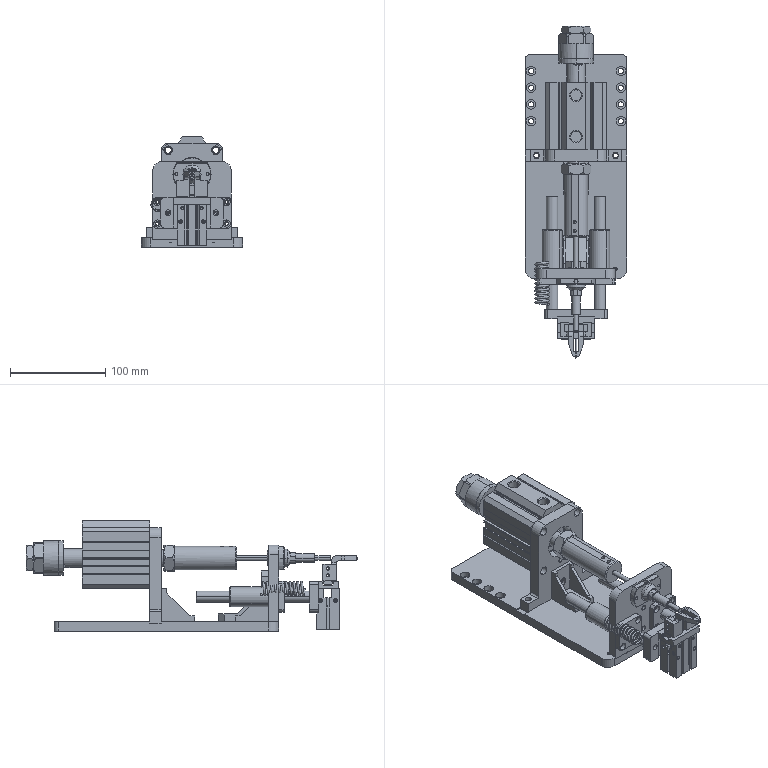Part | SolidWorks | 27 solids | 1468 faces | box 106 x 347.75 x 115.5 mm | volume 813815 mm3 | plane 647 | cylinder 534 | cone 223 | spline 64 | commonest cylinder face diameters 0.4 x45 5 x38 3.3 x32 2 x24 6.5 x24 10 x22